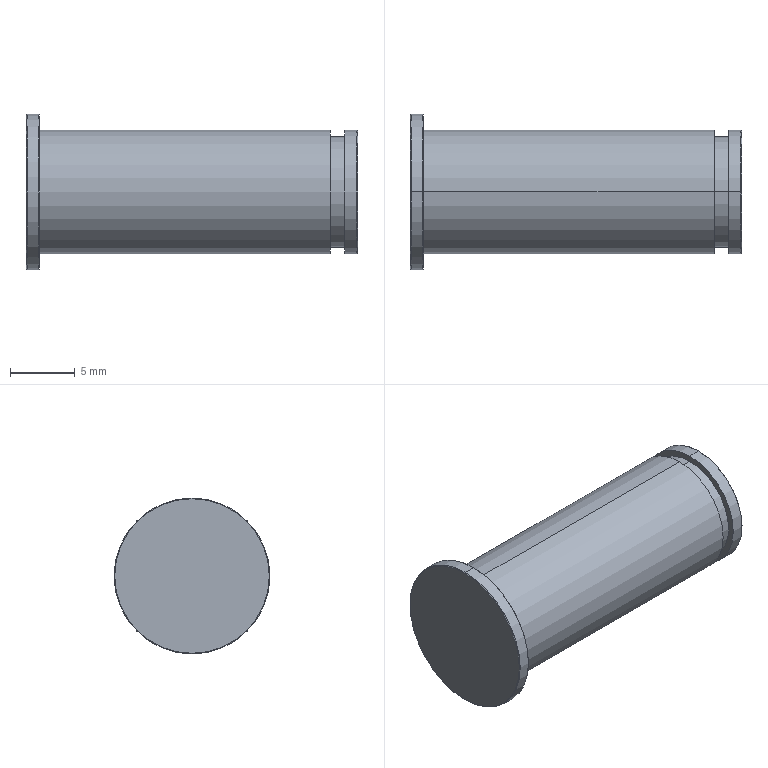Part | SolidWorks | features Chamfer 2, ICE 2, Extrusion 1, Fillet 1 | 1 solid | 21 faces | box 25.5 x 12 x 12 mm | volume 1834 mm3 | cylinder 8 | cone 6 | plane 5 | torus 2 | commonest cylinder face diameters 9.5 x4 8.5 x2 12 x2
STEP:
#1=CARTESIAN_POINT('',(24.45,0.,4.75));
#2=VERTEX_POINT('',#1);
#3=CARTESIAN_POINT('',(24.45,0.,-4.75));
#4=VERTEX_POINT('',#3);
#5=CARTESIAN_POINT('',(24.45,0.,0.));
#6=DIRECTION('',(-1.,0.,0.));
#7=DIRECTION('',(0.,0.,-1.));
#8=AXIS2_PLACEMENT_3D('',#5,#6,#7);
#9=CIRCLE('',#8,4.75);
#10=EDGE_CURVE('',#2,#4,#9,.T.);
#11=ORIENTED_EDGE('',*,*,#10,.T.);
#12=CARTESIAN_POINT('',(23.5,0.,-4.75));
#13=VERTEX_POINT('',#12);
#14=CARTESIAN_POINT('',(24.5,0.,-4.75));
#15=DIRECTION('',(-1.,0.,0.));
#16=VECTOR('',#15,1000.);
#17=LINE('',#14,#16);
#18=EDGE_CURVE('',#4,#13,#17,.T.);
#19=ORIENTED_EDGE('',*,*,#18,.T.);
#20=CARTESIAN_POINT('',(23.5,0.,4.75));
#21=VERTEX_POINT('',#20);
#22=CARTESIAN_POINT('',(23.5,0.,0.));
#23=DIRECTION('',(1.,0.,0.));
#24=DIRECTION('',(0.,0.,-1.));
#25=AXIS2_PLACEMENT_3D('',#22,#23,#24);
#26=CIRCLE('',#25,4.75);
#27=EDGE_CURVE('',#13,#21,#26,.T.);
#28=ORIENTED_EDGE('',*,*,#27,.T.);
#29=CARTESIAN_POINT('',(24.5,0.,4.75));
#30=DIRECTION('',(-1.,0.,0.));
#31=VECTOR('',#30,1000.);
#32=LINE('',#29,#31);
#33=EDGE_CURVE('',#2,#21,#32,.T.);
#34=ORIENTED_EDGE('',*,*,#33,.F.);
#35=EDGE_LOOP('',(#11,#19,#28,#34));
#36=FACE_OUTER_BOUND('',#35,.T.);
#37=CARTESIAN_POINT('',(24.5,0.,0.));
#38=DIRECTION('',(-1.,0.,0.));
#39=DIRECTION('',(0.,0.,1.));
#40=AXIS2_PLACEMENT_3D('',#37,#38,#39);
#41=CYLINDRICAL_SURFACE('',#40,4.75);
#42=ADVANCED_FACE('',(#36),#41,.T.);
#43=CARTESIAN_POINT('',(24.5,0.,-4.7));
#44=VERTEX_POINT('',#43);
#45=CARTESIAN_POINT('',(24.5,0.,4.7));
#46=VERTEX_POINT('',#45);
#47=CARTESIAN_POINT('',(24.5,0.,0.));
#48=DIRECTION('',(1.,0.,0.));
#49=DIRECTION('',(0.,0.,-1.));
#50=AXIS2_PLACEMENT_3D('',#47,#48,#49);
#51=CIRCLE('',#50,4.7);
#52=EDGE_CURVE('',#44,#46,#51,.T.);
#53=ORIENTED_EDGE('',*,*,#52,.F.);
#54=CARTESIAN_POINT('',(24.5,0.,-4.7));
#55=DIRECTION('',(-0.7071,0.,-0.7071));
#56=VECTOR('',#55,1000.);
#57=LINE('',#54,#56);
#58=EDGE_CURVE('',#44,#4,#57,.T.);
#59=ORIENTED_EDGE('',*,*,#58,.T.);
#60=ORIENTED_EDGE('',*,*,#10,.F.);
#61=CARTESIAN_POINT('',(24.5,0.,4.7));
#62=DIRECTION('',(-0.7071,0.,0.7071));
#63=VECTOR('',#62,1000.);
#64=LINE('',#61,#63);
#65=EDGE_CURVE('',#46,#2,#64,.T.);
#66=ORIENTED_EDGE('',*,*,#65,.F.);
#67=EDGE_LOOP('',(#53,#59,#60,#66));
#68=FACE_OUTER_BOUND('',#67,.T.);
#69=CARTESIAN_POINT('',(24.5,0.,0.));
#70=DIRECTION('',(-1.,0.,0.));
#71=DIRECTION('',(0.,0.,1.));
#72=AXIS2_PLACEMENT_3D('',#69,#70,#71);
#73=CONICAL_SURFACE('',#72,4.7,0.7854);
#74=ADVANCED_FACE('',(#68),#73,.T.);
#75=CARTESIAN_POINT('',(22.4,0.,-4.25));
#76=VERTEX_POINT('',#75);
#77=CARTESIAN_POINT('',(22.4,0.,4.25));
#78=VERTEX_POINT('',#77);
#79=CARTESIAN_POINT('',(22.4,0.,0.));
#80=DIRECTION('',(1.,0.,0.));
#81=DIRECTION('',(0.,0.,-1.));
#82=AXIS2_PLACEMENT_3D('',#79,#80,#81);
#83=CIRCLE('',#82,4.25);
#84=EDGE_CURVE('',#76,#78,#83,.T.);
#85=ORIENTED_EDGE('',*,*,#84,.T.);
#86=CARTESIAN_POINT('',(23.5,0.,4.25));
#87=VERTEX_POINT('',#86);
#88=CARTESIAN_POINT('',(22.4,0.,4.25));
#89=DIRECTION('',(1.,0.,0.));
#90=VECTOR('',#89,1000.);
#91=LINE('',#88,#90);
#92=EDGE_CURVE('',#78,#87,#91,.T.);
#93=ORIENTED_EDGE('',*,*,#92,.T.);
#94=CARTESIAN_POINT('',(23.5,0.,-4.25));
#95=VERTEX_POINT('',#94);
#96=CARTESIAN_POINT('',(23.5,0.,0.));
#97=DIRECTION('',(1.,0.,0.));
#98=DIRECTION('',(0.,0.,-1.));
#99=AXIS2_PLACEMENT_3D('',#96,#97,#98);
#100=CIRCLE('',#99,4.25);
#101=EDGE_CURVE('',#95,#87,#100,.T.);
#102=ORIENTED_EDGE('',*,*,#101,.F.);
#103=CARTESIAN_POINT('',(22.4,0.,-4.25));
#104=DIRECTION('',(1.,0.,0.));
#105=VECTOR('',#104,1000.);
#106=LINE('',#103,#105);
#107=EDGE_CURVE('',#76,#95,#106,.T.);
#108=ORIENTED_EDGE('',*,*,#107,.F.);
#109=EDGE_LOOP('',(#85,#93,#102,#108));
#110=FACE_OUTER_BOUND('',#109,.T.);
#111=CARTESIAN_POINT('',(22.4,0.,0.));
#112=DIRECTION('',(1.,0.,0.));
#113=DIRECTION('',(0.,0.,-1.));
#114=AXIS2_PLACEMENT_3D('',#111,#112,#113);
#115=CYLINDRICAL_SURFACE('',#114,4.25);
#116=ADVANCED_FACE('',(#110),#115,.T.);
#117=CARTESIAN_POINT('',(0.,0.,-4.76));
#118=VERTEX_POINT('',#117);
#119=CARTESIAN_POINT('',(0.,0.,4.76));
#120=VERTEX_POINT('',#119);
#121=CARTESIAN_POINT('',(0.,0.,0.));
#122=DIRECTION('',(-1.,0.,0.));
#123=DIRECTION('',(0.,0.,1.));
#124=AXIS2_PLACEMENT_3D('',#121,#122,#123);
#125=CIRCLE('',#124,4.76);
#126=EDGE_CURVE('',#118,#120,#125,.T.);
#127=ORIENTED_EDGE('',*,*,#126,.F.);
#128=CARTESIAN_POINT('',(0.01,0.,-4.75));
#129=VERTEX_POINT('',#128);
#130=CARTESIAN_POINT('',(0.01,0.,-4.76));
#131=DIRECTION('',(0.,1.,0.));
#132=DIRECTION('',(0.,0.,1.));
#133=AXIS2_PLACEMENT_3D('',#130,#131,#132);
#134=CIRCLE('',#133,0.01);
#135=EDGE_CURVE('',#118,#129,#134,.T.);
#136=ORIENTED_EDGE('',*,*,#135,.T.);
#137=CARTESIAN_POINT('',(0.01,0.,4.75));
#138=VERTEX_POINT('',#137);
#139=CARTESIAN_POINT('',(0.01,0.,0.));
#140=DIRECTION('',(1.,0.,0.));
#141=DIRECTION('',(0.,0.,1.));
#142=AXIS2_PLACEMENT_3D('',#139,#140,#141);
#143=CIRCLE('',#142,4.75);
#144=EDGE_CURVE('',#138,#129,#143,.T.);
#145=ORIENTED_EDGE('',*,*,#144,.F.);
#146=CARTESIAN_POINT('',(0.01,0.,4.76));
#147=DIRECTION('',(0.,-1.,0.));
#148=DIRECTION('',(0.,0.,-1.));
#149=AXIS2_PLACEMENT_3D('',#146,#147,#148);
#150=CIRCLE('',#149,0.01);
#151=EDGE_CURVE('',#120,#138,#150,.T.);
#152=ORIENTED_EDGE('',*,*,#151,.F.);
#153=EDGE_LOOP('',(#127,#136,#145,#152));
#154=FACE_OUTER_BOUND('',#153,.T.);
#155=CARTESIAN_POINT('',(0.01,0.,0.));
#156=DIRECTION('',(-1.,0.,0.));
#157=DIRECTION('',(0.,0.,1.));
#158=AXIS2_PLACEMENT_3D('',#155,#156,#157);
#159=TOROIDAL_SURFACE('',#158,4.76,0.01);
#160=ADVANCED_FACE('',(#154),#159,.F.);
#161=CARTESIAN_POINT('',(-1.,0.,5.95));
#162=VERTEX_POINT('',#161);
#163=CARTESIAN_POINT('',(-1.,0.,-5.95));
#164=VERTEX_POINT('',#163);
#165=CARTESIAN_POINT('',(-1.,0.,0.));
#166=DIRECTION('',(-1.,0.,0.));
#167=DIRECTION('',(0.,0.,1.));
#168=AXIS2_PLACEMENT_3D('',#165,#166,#167);
#169=CIRCLE('',#168,5.95);
#170=EDGE_CURVE('',#162,#164,#169,.T.);
#171=ORIENTED_EDGE('',*,*,#170,.F.);
#172=CARTESIAN_POINT('',(-0.95,0.,6.));
#173=VERTEX_POINT('',#172);
#174=CARTESIAN_POINT('',(-1.,0.,5.95));
#175=DIRECTION('',(0.7071,0.,0.7071));
#176=VECTOR('',#175,1000.);
#177=LINE('',#174,#176);
#178=EDGE_CURVE('',#162,#173,#177,.T.);
#179=ORIENTED_EDGE('',*,*,#178,.T.);
#180=CARTESIAN_POINT('',(-0.95,0.,-6.));
#181=VERTEX_POINT('',#180);
#182=CARTESIAN_POINT('',(-0.95,0.,0.));
#183=DIRECTION('',(1.,0.,0.));
#184=DIRECTION('',(0.,0.,1.));
#185=AXIS2_PLACEMENT_3D('',#182,#183,#184);
#186=CIRCLE('',#185,6.);
#187=EDGE_CURVE('',#181,#173,#186,.T.);
#188=ORIENTED_EDGE('',*,*,#187,.F.);
#189=CARTESIAN_POINT('',(-1.,0.,-5.95));
#190=DIRECTION('',(0.7071,0.,-0.7071));
#191=VECTOR('',#190,1000.);
#192=LINE('',#189,#191);
#193=EDGE_CURVE('',#164,#181,#192,.T.);
#194=ORIENTED_EDGE('',*,*,#193,.F.);
#195=EDGE_LOOP('',(#171,#179,#188,#194));
#196=FACE_OUTER_BOUND('',#195,.T.);
#197=CARTESIAN_POINT('',(-1.,0.,0.));
#198=DIRECTION('',(1.,0.,0.));
#199=DIRECTION('',(0.,0.,-1.));
#200=AXIS2_PLACEMENT_3D('',#197,#198,#199);
#201=CONICAL_SURFACE('',#200,5.95,0.7854);
#202=ADVANCED_FACE('',(#196),#201,.T.);
#203=CARTESIAN_POINT('',(0.,0.,-5.95));
#204=VERTEX_POINT('',#203);
#205=CARTESIAN_POINT('',(0.,0.,5.95));
#206=VERTEX_POINT('',#205);
#207=CARTESIAN_POINT('',(0.,0.,0.));
#208=DIRECTION('',(1.,0.,0.));
#209=DIRECTION('',(0.,0.,1.));
#210=AXIS2_PLACEMENT_3D('',#207,#208,#209);
#211=CIRCLE('',#210,5.95);
#212=EDGE_CURVE('',#204,#206,#211,.T.);
#213=ORIENTED_EDGE('',*,*,#212,.F.);
#214=CARTESIAN_POINT('',(-0.05,0.,-6.));
#215=VERTEX_POINT('',#214);
#216=CARTESIAN_POINT('',(-0.05,0.,-6.));
#217=DIRECTION('',(-0.7071,0.,-0.7071));
#218=VECTOR('',#217,1000.);
#219=LINE('',#216,#218);
#220=EDGE_CURVE('',#204,#215,#219,.T.);
#221=ORIENTED_EDGE('',*,*,#220,.T.);
#222=CARTESIAN_POINT('',(-0.05,0.,6.));
#223=VERTEX_POINT('',#222);
#224=CARTESIAN_POINT('',(-0.05,0.,0.));
#225=DIRECTION('',(-1.,0.,0.));
#226=DIRECTION('',(0.,0.,1.));
#227=AXIS2_PLACEMENT_3D('',#224,#225,#226);
#228=CIRCLE('',#227,6.);
#229=EDGE_CURVE('',#223,#215,#228,.T.);
#230=ORIENTED_EDGE('',*,*,#229,.F.);
#231=CARTESIAN_POINT('',(-0.05,0.,6.));
#232=DIRECTION('',(-0.7071,0.,0.7071));
#233=VECTOR('',#232,1000.);
#234=LINE('',#231,#233);
#235=EDGE_CURVE('',#206,#223,#234,.T.);
#236=ORIENTED_EDGE('',*,*,#235,.F.);
#237=EDGE_LOOP('',(#213,#221,#230,#236));
#238=FACE_OUTER_BOUND('',#237,.T.);
#239=CARTESIAN_POINT('',(-0.05,0.,0.));
#240=DIRECTION('',(-1.,0.,0.));
#241=DIRECTION('',(0.,0.,1.));
#242=AXIS2_PLACEMENT_3D('',#239,#240,#241);
#243=CONICAL_SURFACE('',#242,6.,0.7854);
#244=ADVANCED_FACE('',(#238),#243,.T.);
#245=ORIENTED_EDGE('',*,*,#187,.T.);
#246=CARTESIAN_POINT('',(-1.,0.,6.));
#247=DIRECTION('',(1.,0.,0.));
#248=VECTOR('',#247,1000.);
#249=LINE('',#246,#248);
#250=EDGE_CURVE('',#173,#223,#249,.T.);
#251=ORIENTED_EDGE('',*,*,#250,.T.);
#252=ORIENTED_EDGE('',*,*,#229,.T.);
#253=CARTESIAN_POINT('',(-1.,0.,-6.));
#254=DIRECTION('',(1.,0.,0.));
#255=VECTOR('',#254,1000.);
#256=LINE('',#253,#255);
#257=EDGE_CURVE('',#181,#215,#256,.T.);
#258=ORIENTED_EDGE('',*,*,#257,.F.);
#259=EDGE_LOOP('',(#245,#251,#252,#258));
#260=FACE_OUTER_BOUND('',#259,.T.);
#261=CARTESIAN_POINT('',(-1.,0.,0.));
#262=DIRECTION('',(1.,0.,0.));
#263=DIRECTION('',(0.,0.,-1.));
#264=AXIS2_PLACEMENT_3D('',#261,#262,#263);
#265=CYLINDRICAL_SURFACE('',#264,6.);
#266=ADVANCED_FACE('',(#260),#265,.T.);
#267=CARTESIAN_POINT('',(22.4,0.,-4.75));
#268=VERTEX_POINT('',#267);
#269=CARTESIAN_POINT('',(22.4,0.,4.75));
#270=VERTEX_POINT('',#269);
#271=CARTESIAN_POINT('',(22.4,0.,0.));
#272=DIRECTION('',(1.,0.,0.));
#273=DIRECTION('',(0.,0.,-1.));
#274=AXIS2_PLACEMENT_3D('',#271,#272,#273);
#275=CIRCLE('',#274,4.75);
#276=EDGE_CURVE('',#268,#270,#275,.T.);
#277=ORIENTED_EDGE('',*,*,#276,.F.);
#278=CARTESIAN_POINT('',(24.5,0.,-4.75));
#279=DIRECTION('',(-1.,0.,0.));
#280=VECTOR('',#279,1000.);
#281=LINE('',#278,#280);
#282=EDGE_CURVE('',#268,#129,#281,.T.);
#283=ORIENTED_EDGE('',*,*,#282,.T.);
#284=CARTESIAN_POINT('',(0.01,0.,0.));
#285=DIRECTION('',(1.,0.,0.));
#286=DIRECTION('',(0.,0.,1.));
#287=AXIS2_PLACEMENT_3D('',#284,#285,#286);
#288=CIRCLE('',#287,4.75);
#289=EDGE_CURVE('',#129,#138,#288,.T.);
#290=ORIENTED_EDGE('',*,*,#289,.T.);
#291=CARTESIAN_POINT('',(24.5,0.,4.75));
#292=DIRECTION('',(-1.,0.,0.));
#293=VECTOR('',#292,1000.);
#294=LINE('',#291,#293);
#295=EDGE_CURVE('',#270,#138,#294,.T.);
#296=ORIENTED_EDGE('',*,*,#295,.F.);
#297=EDGE_LOOP('',(#277,#283,#290,#296));
#298=FACE_OUTER_BOUND('',#297,.T.);
#299=CARTESIAN_POINT('',(24.5,0.,0.));
#300=DIRECTION('',(-1.,0.,0.));
#301=DIRECTION('',(0.,0.,1.));
#302=AXIS2_PLACEMENT_3D('',#299,#300,#301);
#303=CYLINDRICAL_SURFACE('',#302,4.75);
#304=ADVANCED_FACE('',(#298),#303,.T.);
#305=ORIENTED_EDGE('',*,*,#282,.F.);
#306=CARTESIAN_POINT('',(22.4,0.,0.));
#307=DIRECTION('',(1.,0.,0.));
#308=DIRECTION('',(0.,0.,-1.));
#309=AXIS2_PLACEMENT_3D('',#306,#307,#308);
#310=CIRCLE('',#309,4.75);
#311=EDGE_CURVE('',#270,#268,#310,.T.);
#312=ORIENTED_EDGE('',*,*,#311,.F.);
#313=ORIENTED_EDGE('',*,*,#295,.T.);
#314=ORIENTED_EDGE('',*,*,#144,.T.);
#315=EDGE_LOOP('',(#305,#312,#313,#314));
#316=FACE_OUTER_BOUND('',#315,.T.);
#317=CARTESIAN_POINT('',(24.5,0.,0.));
#318=DIRECTION('',(-1.,0.,0.));
#319=DIRECTION('',(0.,0.,1.));
#320=AXIS2_PLACEMENT_3D('',#317,#318,#319);
#321=CYLINDRICAL_SURFACE('',#320,4.75);
#322=ADVANCED_FACE('',(#316),#321,.T.);
#323=CARTESIAN_POINT('',(0.,0.,0.));
#324=DIRECTION('',(-1.,0.,0.));
#325=DIRECTION('',(0.,0.,1.));
#326=AXIS2_PLACEMENT_3D('',#323,#324,#325);
#327=CIRCLE('',#326,4.76);
#328=EDGE_CURVE('',#120,#118,#327,.T.);
#329=ORIENTED_EDGE('',*,*,#328,.T.);
#330=ORIENTED_EDGE('',*,*,#126,.T.);
#331=EDGE_LOOP('',(#329,#330));
#332=FACE_BOUND('',#331,.T.);
#333=CARTESIAN_POINT('',(0.,0.,0.));
#334=DIRECTION('',(1.,0.,0.));
#335=DIRECTION('',(0.,0.,1.));
#336=AXIS2_PLACEMENT_3D('',#333,#334,#335);
#337=CIRCLE('',#336,5.95);
#338=EDGE_CURVE('',#206,#204,#337,.T.);
#339=ORIENTED_EDGE('',*,*,#338,.T.);
#340=ORIENTED_EDGE('',*,*,#212,.T.);
#341=EDGE_LOOP('',(#339,#340));
#342=FACE_OUTER_BOUND('',#341,.T.);
#343=CARTESIAN_POINT('',(0.,0.,0.));
#344=DIRECTION('',(-1.,0.,0.));
#345=DIRECTION('',(0.,0.,1.));
#346=AXIS2_PLACEMENT_3D('',#343,#344,#345);
#347=PLANE('',#346);
#348=ADVANCED_FACE('',(#332,#342),#347,.F.);
#349=ORIENTED_EDGE('',*,*,#250,.F.);
#350=CARTESIAN_POINT('',(-0.95,0.,0.));
#351=DIRECTION('',(1.,0.,0.));
#352=DIRECTION('',(0.,0.,1.));
#353=AXIS2_PLACEMENT_3D('',#350,#351,#352);
#354=CIRCLE('',#353,6.);
#355=EDGE_CURVE('',#173,#181,#354,.T.);
#356=ORIENTED_EDGE('',*,*,#355,.T.);
#357=ORIENTED_EDGE('',*,*,#257,.T.);
#358=CARTESIAN_POINT('',(-0.05,0.,0.));
#359=DIRECTION('',(-1.,0.,0.));
#360=DIRECTION('',(0.,0.,1.));
#361=AXIS2_PLACEMENT_3D('',#358,#359,#360);
#362=CIRCLE('',#361,6.);
#363=EDGE_CURVE('',#215,#223,#362,.T.);
#364=ORIENTED_EDGE('',*,*,#363,.T.);
#365=EDGE_LOOP('',(#349,#356,#357,#364));
#366=FACE_OUTER_BOUND('',#365,.T.);
#367=CARTESIAN_POINT('',(-1.,0.,0.));
#368=DIRECTION('',(1.,0.,0.));
#369=DIRECTION('',(0.,0.,-1.));
#370=AXIS2_PLACEMENT_3D('',#367,#368,#369);
#371=CYLINDRICAL_SURFACE('',#370,6.);
#372=ADVANCED_FACE('',(#366),#371,.T.);
#373=CARTESIAN_POINT('',(-1.,0.,0.));
#374=DIRECTION('',(-1.,0.,0.));
#375=DIRECTION('',(0.,0.,1.));
#376=AXIS2_PLACEMENT_3D('',#373,#374,#375);
#377=CIRCLE('',#376,5.95);
#378=EDGE_CURVE('',#164,#162,#377,.T.);
#379=ORIENTED_EDGE('',*,*,#378,.T.);
#380=ORIENTED_EDGE('',*,*,#170,.T.);
#381=EDGE_LOOP('',(#379,#380));
#382=FACE_OUTER_BOUND('',#381,.T.);
#383=CARTESIAN_POINT('',(-1.,0.,0.));
#384=DIRECTION('',(-1.,0.,0.));
#385=DIRECTION('',(0.,0.,1.));
#386=AXIS2_PLACEMENT_3D('',#383,#384,#385);
#387=PLANE('',#386);
#388=ADVANCED_FACE('',(#382),#387,.T.);
#389=ORIENTED_EDGE('',*,*,#220,.F.);
#390=ORIENTED_EDGE('',*,*,#338,.F.);
#391=ORIENTED_EDGE('',*,*,#235,.T.);
#392=ORIENTED_EDGE('',*,*,#363,.F.);
#393=EDGE_LOOP('',(#389,#390,#391,#392));
#394=FACE_OUTER_BOUND('',#393,.T.);
#395=CARTESIAN_POINT('',(-0.05,0.,0.));
#396=DIRECTION('',(-1.,0.,0.));
#397=DIRECTION('',(0.,0.,1.));
#398=AXIS2_PLACEMENT_3D('',#395,#396,#397);
#399=CONICAL_SURFACE('',#398,6.,0.7854);
#400=ADVANCED_FACE('',(#394),#399,.T.);
#401=ORIENTED_EDGE('',*,*,#178,.F.);
#402=ORIENTED_EDGE('',*,*,#378,.F.);
#403=ORIENTED_EDGE('',*,*,#193,.T.);
#404=ORIENTED_EDGE('',*,*,#355,.F.);
#405=EDGE_LOOP('',(#401,#402,#403,#404));
#406=FACE_OUTER_BOUND('',#405,.T.);
#407=CARTESIAN_POINT('',(-1.,0.,0.));
#408=DIRECTION('',(1.,0.,0.));
#409=DIRECTION('',(0.,0.,-1.));
#410=AXIS2_PLACEMENT_3D('',#407,#408,#409);
#411=CONICAL_SURFACE('',#410,5.95,0.7854);
#412=ADVANCED_FACE('',(#406),#411,.T.);
#413=ORIENTED_EDGE('',*,*,#135,.F.);
#414=ORIENTED_EDGE('',*,*,#328,.F.);
#415=ORIENTED_EDGE('',*,*,#151,.T.);
#416=ORIENTED_EDGE('',*,*,#289,.F.);
#417=EDGE_LOOP('',(#413,#414,#415,#416));
#418=FACE_OUTER_BOUND('',#417,.T.);
#419=CARTESIAN_POINT('',(0.01,0.,0.));
#420=DIRECTION('',(-1.,0.,0.));
#421=DIRECTION('',(0.,0.,1.));
#422=AXIS2_PLACEMENT_3D('',#419,#420,#421);
#423=TOROIDAL_SURFACE('',#422,4.76,0.01);
#424=ADVANCED_FACE('',(#418),#423,.F.);
#425=ORIENTED_EDGE('',*,*,#84,.F.);
#426=CARTESIAN_POINT('',(22.4,0.,0.));
#427=DIRECTION('',(1.,0.,0.));
#428=DIRECTION('',(0.,0.,-1.));
#429=AXIS2_PLACEMENT_3D('',#426,#427,#428);
#430=CIRCLE('',#429,4.25);
#431=EDGE_CURVE('',#78,#76,#430,.T.);
#432=ORIENTED_EDGE('',*,*,#431,.F.);
#433=EDGE_LOOP('',(#425,#432));
#434=FACE_BOUND('',#433,.T.);
#435=ORIENTED_EDGE('',*,*,#311,.T.);
#436=ORIENTED_EDGE('',*,*,#276,.T.);
#437=EDGE_LOOP('',(#435,#436));
#438=FACE_OUTER_BOUND('',#437,.T.);
#439=CARTESIAN_POINT('',(22.4,0.,0.));
#440=DIRECTION('',(1.,0.,0.));
#441=DIRECTION('',(0.,0.,-1.));
#442=AXIS2_PLACEMENT_3D('',#439,#440,#441);
#443=PLANE('',#442);
#444=ADVANCED_FACE('',(#434,#438),#443,.T.);
#445=ORIENTED_EDGE('',*,*,#101,.T.);
#446=CARTESIAN_POINT('',(23.5,0.,0.));
#447=DIRECTION('',(1.,0.,0.));
#448=DIRECTION('',(0.,0.,-1.));
#449=AXIS2_PLACEMENT_3D('',#446,#447,#448);
#450=CIRCLE('',#449,4.25);
#451=EDGE_CURVE('',#87,#95,#450,.T.);
#452=ORIENTED_EDGE('',*,*,#451,.T.);
#453=EDGE_LOOP('',(#445,#452));
#454=FACE_BOUND('',#453,.T.);
#455=CARTESIAN_POINT('',(23.5,0.,0.));
#456=DIRECTION('',(1.,0.,0.));
#457=DIRECTION('',(0.,0.,-1.));
#458=AXIS2_PLACEMENT_3D('',#455,#456,#457);
#459=CIRCLE('',#458,4.75);
#460=EDGE_CURVE('',#21,#13,#459,.T.);
#461=ORIENTED_EDGE('',*,*,#460,.F.);
#462=ORIENTED_EDGE('',*,*,#27,.F.);
#463=EDGE_LOOP('',(#461,#462));
#464=FACE_OUTER_BOUND('',#463,.T.);
#465=CARTESIAN_POINT('',(23.5,0.,0.));
#466=DIRECTION('',(1.,0.,0.));
#467=DIRECTION('',(0.,0.,-1.));
#468=AXIS2_PLACEMENT_3D('',#465,#466,#467);
#469=PLANE('',#468);
#470=ADVANCED_FACE('',(#454,#464),#469,.F.);
#471=ORIENTED_EDGE('',*,*,#92,.F.);
#472=ORIENTED_EDGE('',*,*,#431,.T.);
#473=ORIENTED_EDGE('',*,*,#107,.T.);
#474=ORIENTED_EDGE('',*,*,#451,.F.);
#475=EDGE_LOOP('',(#471,#472,#473,#474));
#476=FACE_OUTER_BOUND('',#475,.T.);
#477=CARTESIAN_POINT('',(22.4,0.,0.));
#478=DIRECTION('',(1.,0.,0.));
#479=DIRECTION('',(0.,0.,-1.));
#480=AXIS2_PLACEMENT_3D('',#477,#478,#479);
#481=CYLINDRICAL_SURFACE('',#480,4.25);
#482=ADVANCED_FACE('',(#476),#481,.T.);
#483=CARTESIAN_POINT('',(24.5,0.,0.));
#484=DIRECTION('',(1.,0.,0.));
#485=DIRECTION('',(0.,0.,-1.));
#486=AXIS2_PLACEMENT_3D('',#483,#484,#485);
#487=CIRCLE('',#486,4.7);
#488=EDGE_CURVE('',#46,#44,#487,.T.);
#489=ORIENTED_EDGE('',*,*,#488,.T.);
#490=ORIENTED_EDGE('',*,*,#52,.T.);
#491=EDGE_LOOP('',(#489,#490));
#492=FACE_OUTER_BOUND('',#491,.T.);
#493=CARTESIAN_POINT('',(24.5,0.,0.));
#494=DIRECTION('',(1.,0.,0.));
#495=DIRECTION('',(0.,0.,-1.));
#496=AXIS2_PLACEMENT_3D('',#493,#494,#495);
#497=PLANE('',#496);
#498=ADVANCED_FACE('',(#492),#497,.T.);
#499=ORIENTED_EDGE('',*,*,#58,.F.);
#500=ORIENTED_EDGE('',*,*,#488,.F.);
#501=ORIENTED_EDGE('',*,*,#65,.T.);
#502=CARTESIAN_POINT('',(24.45,0.,0.));
#503=DIRECTION('',(-1.,0.,0.));
#504=DIRECTION('',(0.,0.,-1.));
#505=AXIS2_PLACEMENT_3D('',#502,#503,#504);
#506=CIRCLE('',#505,4.75);
#507=EDGE_CURVE('',#4,#2,#506,.T.);
#508=ORIENTED_EDGE('',*,*,#507,.F.);
#509=EDGE_LOOP('',(#499,#500,#501,#508));
#510=FACE_OUTER_BOUND('',#509,.T.);
#511=CARTESIAN_POINT('',(24.5,0.,0.));
#512=DIRECTION('',(-1.,0.,0.));
#513=DIRECTION('',(0.,0.,1.));
#514=AXIS2_PLACEMENT_3D('',#511,#512,#513);
#515=CONICAL_SURFACE('',#514,4.7,0.7854);
#516=ADVANCED_FACE('',(#510),#515,.T.);
#517=ORIENTED_EDGE('',*,*,#18,.F.);
#518=ORIENTED_EDGE('',*,*,#507,.T.);
#519=ORIENTED_EDGE('',*,*,#33,.T.);
#520=ORIENTED_EDGE('',*,*,#460,.T.);
#521=EDGE_LOOP('',(#517,#518,#519,#520));
#522=FACE_OUTER_BOUND('',#521,.T.);
#523=CARTESIAN_POINT('',(24.5,0.,0.));
#524=DIRECTION('',(-1.,0.,0.));
#525=DIRECTION('',(0.,0.,1.));
#526=AXIS2_PLACEMENT_3D('',#523,#524,#525);
#527=CYLINDRICAL_SURFACE('',#526,4.75);
#528=ADVANCED_FACE('',(#522),#527,.T.);
#529=CLOSED_SHELL('',(#42,#74,#116,#160,#202,#244,#266,#304,#322,#348,#372,#388,#400,#412,#424,#444,#470,#482,#498,#516,#528));
#530=MANIFOLD_SOLID_BREP('',#529);
#531=CARTESIAN_POINT('',(0.,0.,0.));
#532=DIRECTION('',(0.,0.,1.));
#533=DIRECTION('',(1.,0.,0.));
#534=AXIS2_PLACEMENT_3D('',#531,#532,#533);
#535=(LENGTH_UNIT()NAMED_UNIT(*)SI_UNIT(.MILLI.,.METRE.));
#536=UNCERTAINTY_MEASURE_WITH_UNIT(LENGTH_MEASURE(0.00001),#535,'','');
#537=(NAMED_UNIT(*)PLANE_ANGLE_UNIT()SI_UNIT($,.RADIAN.));
#538=(NAMED_UNIT(*)SI_UNIT($,.STERADIAN.)SOLID_ANGLE_UNIT());
#539=(GEOMETRIC_REPRESENTATION_CONTEXT(3)GLOBAL_UNCERTAINTY_ASSIGNED_CONTEXT((#536))GLOBAL_UNIT_ASSIGNED_CONTEXT((#535,#537,#538))REPRESENTATION_CONTEXT('',''));
#540=ADVANCED_BREP_SHAPE_REPRESENTATION('',(#530,#534),#539);